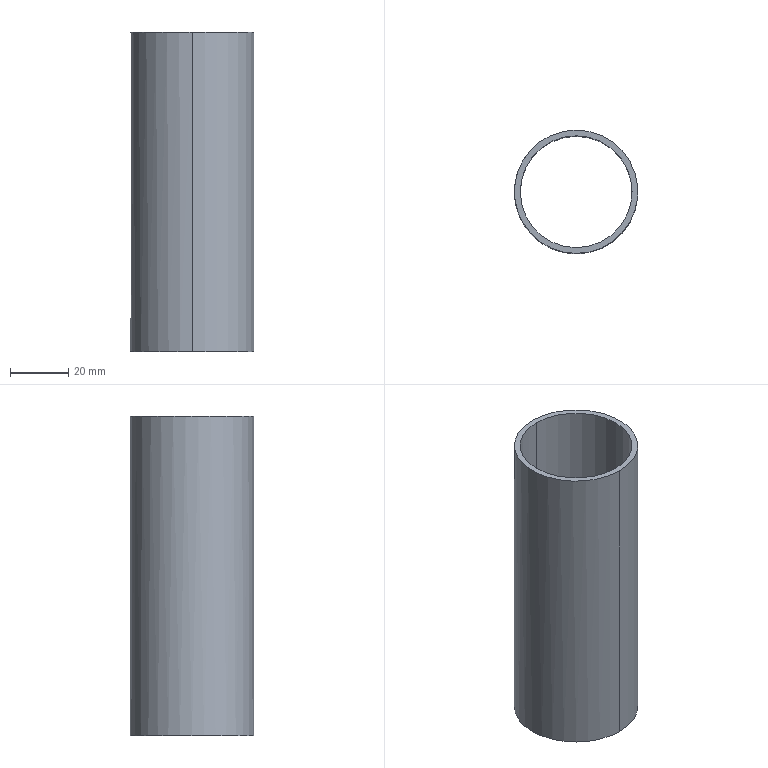Part | NX | features MYKP38-200_3 2 | 1 solid | 6 faces | box 42.5 x 42.5 x 110 mm | volume 27992 mm3 | cylinder 4 | plane 2 | commonest cylinder face diameters 38.5 x2 42.5 x2
STEP:
#1=CARTESIAN_POINT('',(1759.977,-291.155,-110.001));
#2=VERTEX_POINT('',#1);
#3=CARTESIAN_POINT('',(1738.727,-312.405,-110.001));
#4=VERTEX_POINT('',#3);
#5=CARTESIAN_POINT('',(1759.977,-312.405,-110.001));
#6=DIRECTION('',(0.,0.,1.));
#7=DIRECTION('',(0.,1.,0.));
#8=AXIS2_PLACEMENT_3D('',#5,#6,#7);
#9=CIRCLE('',#8,21.25);
#10=EDGE_CURVE('',#2,#4,#9,.T.);
#11=ORIENTED_EDGE('',*,*,#10,.F.);
#12=CARTESIAN_POINT('',(1759.977,-333.655,-110.001));
#13=VERTEX_POINT('',#12);
#14=CARTESIAN_POINT('',(1759.977,-312.405,-110.001));
#15=DIRECTION('',(0.,0.,1.));
#16=DIRECTION('',(0.,-1.,0.));
#17=AXIS2_PLACEMENT_3D('',#14,#15,#16);
#18=CIRCLE('',#17,21.25);
#19=EDGE_CURVE('',#13,#2,#18,.T.);
#20=ORIENTED_EDGE('',*,*,#19,.F.);
#21=CARTESIAN_POINT('',(1759.977,-312.405,-110.001));
#22=DIRECTION('',(0.,0.,1.));
#23=DIRECTION('',(-1.,0.,0.));
#24=AXIS2_PLACEMENT_3D('',#21,#22,#23);
#25=CIRCLE('',#24,21.25);
#26=EDGE_CURVE('',#4,#13,#25,.T.);
#27=ORIENTED_EDGE('',*,*,#26,.F.);
#28=EDGE_LOOP('',(#11,#20,#27));
#29=FACE_BOUND('',#28,.T.);
#30=CARTESIAN_POINT('',(1740.727,-312.405,-110.001));
#31=VERTEX_POINT('',#30);
#32=CARTESIAN_POINT('',(1759.977,-293.155,-110.001));
#33=VERTEX_POINT('',#32);
#34=CARTESIAN_POINT('',(1759.977,-312.405,-110.001));
#35=DIRECTION('',(0.,0.,-1.));
#36=DIRECTION('',(-1.,0.,0.));
#37=AXIS2_PLACEMENT_3D('',#34,#35,#36);
#38=CIRCLE('',#37,19.25);
#39=EDGE_CURVE('',#31,#33,#38,.T.);
#40=ORIENTED_EDGE('',*,*,#39,.F.);
#41=CARTESIAN_POINT('',(1759.977,-331.655,-110.001));
#42=VERTEX_POINT('',#41);
#43=CARTESIAN_POINT('',(1759.977,-312.405,-110.001));
#44=DIRECTION('',(0.,0.,-1.));
#45=DIRECTION('',(0.,-1.,0.));
#46=AXIS2_PLACEMENT_3D('',#43,#44,#45);
#47=CIRCLE('',#46,19.25);
#48=EDGE_CURVE('',#42,#31,#47,.T.);
#49=ORIENTED_EDGE('',*,*,#48,.F.);
#50=CARTESIAN_POINT('',(1779.227,-312.405,-110.001));
#51=VERTEX_POINT('',#50);
#52=CARTESIAN_POINT('',(1759.977,-312.405,-110.001));
#53=DIRECTION('',(0.,0.,-1.));
#54=DIRECTION('',(1.,0.,0.));
#55=AXIS2_PLACEMENT_3D('',#52,#53,#54);
#56=CIRCLE('',#55,19.25);
#57=EDGE_CURVE('',#51,#42,#56,.T.);
#58=ORIENTED_EDGE('',*,*,#57,.F.);
#59=CARTESIAN_POINT('',(1759.977,-312.405,-110.001));
#60=DIRECTION('',(0.,0.,-1.));
#61=DIRECTION('',(0.,1.,0.));
#62=AXIS2_PLACEMENT_3D('',#59,#60,#61);
#63=CIRCLE('',#62,19.25);
#64=EDGE_CURVE('',#33,#51,#63,.T.);
#65=ORIENTED_EDGE('',*,*,#64,.F.);
#66=EDGE_LOOP('',(#40,#49,#58,#65));
#67=FACE_BOUND('',#66,.T.);
#68=CARTESIAN_POINT('',(1736.227,-312.405,-110.001));
#69=DIRECTION('',(0.,0.,1.));
#70=DIRECTION('',(0.,-1.,0.));
#71=AXIS2_PLACEMENT_3D('',#68,#69,#70);
#72=PLANE('',#71);
#73=ADVANCED_FACE('',(#29,#67),#72,.F.);
#74=CARTESIAN_POINT('',(1759.977,-291.155,-0.0008318));
#75=VERTEX_POINT('',#74);
#76=CARTESIAN_POINT('',(1759.977,-291.155,-70.001));
#77=DIRECTION('',(0.,0.,-1.));
#78=VECTOR('',#77,1000.);
#79=LINE('',#76,#78);
#80=EDGE_CURVE('',#75,#2,#79,.T.);
#81=ORIENTED_EDGE('',*,*,#80,.F.);
#82=CARTESIAN_POINT('',(1759.977,-333.655,-0.0008318));
#83=VERTEX_POINT('',#82);
#84=CARTESIAN_POINT('',(1759.977,-312.405,-0.0008318));
#85=DIRECTION('',(0.,0.,-1.));
#86=DIRECTION('',(0.,1.,0.));
#87=AXIS2_PLACEMENT_3D('',#84,#85,#86);
#88=CIRCLE('',#87,21.25);
#89=EDGE_CURVE('',#75,#83,#88,.T.);
#90=ORIENTED_EDGE('',*,*,#89,.T.);
#91=CARTESIAN_POINT('',(1759.977,-333.655,-4094.001));
#92=DIRECTION('',(0.,0.,-1.));
#93=VECTOR('',#92,1000.);
#94=LINE('',#91,#93);
#95=EDGE_CURVE('',#13,#83,#94,.F.);
#96=ORIENTED_EDGE('',*,*,#95,.F.);
#97=ORIENTED_EDGE('',*,*,#19,.T.);
#98=EDGE_LOOP('',(#81,#90,#96,#97));
#99=FACE_BOUND('',#98,.T.);
#100=CARTESIAN_POINT('',(1759.977,-312.405,49.999));
#101=DIRECTION('',(0.,0.,-1.));
#102=DIRECTION('',(-1.,0.,0.));
#103=AXIS2_PLACEMENT_3D('',#100,#101,#102);
#104=CYLINDRICAL_SURFACE('',#103,21.25);
#105=ADVANCED_FACE('',(#99),#104,.T.);
#106=CARTESIAN_POINT('',(1759.977,-293.155,-0.0008318));
#107=VERTEX_POINT('',#106);
#108=CARTESIAN_POINT('',(1759.977,-293.155,-70.001));
#109=DIRECTION('',(0.,0.,-1.));
#110=VECTOR('',#109,1000.);
#111=LINE('',#108,#110);
#112=EDGE_CURVE('',#33,#107,#111,.F.);
#113=ORIENTED_EDGE('',*,*,#112,.T.);
#114=CARTESIAN_POINT('',(1759.977,-331.655,-0.0008318));
#115=VERTEX_POINT('',#114);
#116=CARTESIAN_POINT('',(1759.977,-312.405,-0.0008318));
#117=DIRECTION('',(0.,0.,1.));
#118=DIRECTION('',(0.,1.,0.));
#119=AXIS2_PLACEMENT_3D('',#116,#117,#118);
#120=CIRCLE('',#119,19.25);
#121=EDGE_CURVE('',#107,#115,#120,.T.);
#122=ORIENTED_EDGE('',*,*,#121,.T.);
#123=CARTESIAN_POINT('',(1759.977,-331.655,-4094.001));
#124=DIRECTION('',(0.,0.,-1.));
#125=VECTOR('',#124,1000.);
#126=LINE('',#123,#125);
#127=EDGE_CURVE('',#115,#42,#126,.T.);
#128=ORIENTED_EDGE('',*,*,#127,.T.);
#129=ORIENTED_EDGE('',*,*,#48,.T.);
#130=ORIENTED_EDGE('',*,*,#39,.T.);
#131=EDGE_LOOP('',(#113,#122,#128,#129,#130));
#132=FACE_BOUND('',#131,.T.);
#133=CARTESIAN_POINT('',(1759.977,-312.405,49.999));
#134=DIRECTION('',(0.,0.,-1.));
#135=DIRECTION('',(-1.,0.,0.));
#136=AXIS2_PLACEMENT_3D('',#133,#134,#135);
#137=CYLINDRICAL_SURFACE('',#136,19.25);
#138=ADVANCED_FACE('',(#132),#137,.F.);
#139=ORIENTED_EDGE('',*,*,#95,.T.);
#140=CARTESIAN_POINT('',(1759.977,-312.405,-0.0008318));
#141=DIRECTION('',(0.,0.,-1.));
#142=DIRECTION('',(0.,-1.,0.));
#143=AXIS2_PLACEMENT_3D('',#140,#141,#142);
#144=CIRCLE('',#143,21.25);
#145=EDGE_CURVE('',#83,#75,#144,.T.);
#146=ORIENTED_EDGE('',*,*,#145,.T.);
#147=ORIENTED_EDGE('',*,*,#80,.T.);
#148=ORIENTED_EDGE('',*,*,#10,.T.);
#149=ORIENTED_EDGE('',*,*,#26,.T.);
#150=EDGE_LOOP('',(#139,#146,#147,#148,#149));
#151=FACE_BOUND('',#150,.T.);
#152=CARTESIAN_POINT('',(1759.977,-312.405,49.999));
#153=DIRECTION('',(0.,0.,-1.));
#154=DIRECTION('',(-1.,0.,0.));
#155=AXIS2_PLACEMENT_3D('',#152,#153,#154);
#156=CYLINDRICAL_SURFACE('',#155,21.25);
#157=ADVANCED_FACE('',(#151),#156,.T.);
#158=ORIENTED_EDGE('',*,*,#127,.F.);
#159=CARTESIAN_POINT('',(1759.977,-312.405,-0.0008318));
#160=DIRECTION('',(0.,0.,1.));
#161=DIRECTION('',(0.,-1.,0.));
#162=AXIS2_PLACEMENT_3D('',#159,#160,#161);
#163=CIRCLE('',#162,19.25);
#164=EDGE_CURVE('',#115,#107,#163,.T.);
#165=ORIENTED_EDGE('',*,*,#164,.T.);
#166=ORIENTED_EDGE('',*,*,#112,.F.);
#167=ORIENTED_EDGE('',*,*,#64,.T.);
#168=ORIENTED_EDGE('',*,*,#57,.T.);
#169=EDGE_LOOP('',(#158,#165,#166,#167,#168));
#170=FACE_BOUND('',#169,.T.);
#171=CARTESIAN_POINT('',(1759.977,-312.405,49.999));
#172=DIRECTION('',(0.,0.,-1.));
#173=DIRECTION('',(-1.,0.,0.));
#174=AXIS2_PLACEMENT_3D('',#171,#172,#173);
#175=CYLINDRICAL_SURFACE('',#174,19.25);
#176=ADVANCED_FACE('',(#170),#175,.F.);
#177=ORIENTED_EDGE('',*,*,#145,.F.);
#178=ORIENTED_EDGE('',*,*,#89,.F.);
#179=EDGE_LOOP('',(#177,#178));
#180=FACE_BOUND('',#179,.T.);
#181=ORIENTED_EDGE('',*,*,#164,.F.);
#182=ORIENTED_EDGE('',*,*,#121,.F.);
#183=EDGE_LOOP('',(#181,#182));
#184=FACE_BOUND('',#183,.T.);
#185=CARTESIAN_POINT('',(1723.477,-312.405,-0.0008318));
#186=DIRECTION('',(0.,0.,-1.));
#187=DIRECTION('',(1.,0.,0.));
#188=AXIS2_PLACEMENT_3D('',#185,#186,#187);
#189=PLANE('',#188);
#190=ADVANCED_FACE('',(#180,#184),#189,.F.);
#191=CLOSED_SHELL('',(#73,#105,#138,#157,#176,#190));
#192=MANIFOLD_SOLID_BREP('',#191);
#193=(LENGTH_UNIT()NAMED_UNIT(*)SI_UNIT(.MILLI.,.METRE.));
#194=UNCERTAINTY_MEASURE_WITH_UNIT(LENGTH_MEASURE(0.00001),#193,'','');
#195=(NAMED_UNIT(*)PLANE_ANGLE_UNIT()SI_UNIT($,.RADIAN.));
#196=(NAMED_UNIT(*)SI_UNIT($,.STERADIAN.)SOLID_ANGLE_UNIT());
#197=(GEOMETRIC_REPRESENTATION_CONTEXT(3)GLOBAL_UNCERTAINTY_ASSIGNED_CONTEXT((#194))GLOBAL_UNIT_ASSIGNED_CONTEXT((#193,#195,#196))REPRESENTATION_CONTEXT('',''));
#198=ADVANCED_BREP_SHAPE_REPRESENTATION('',(#192),#197);